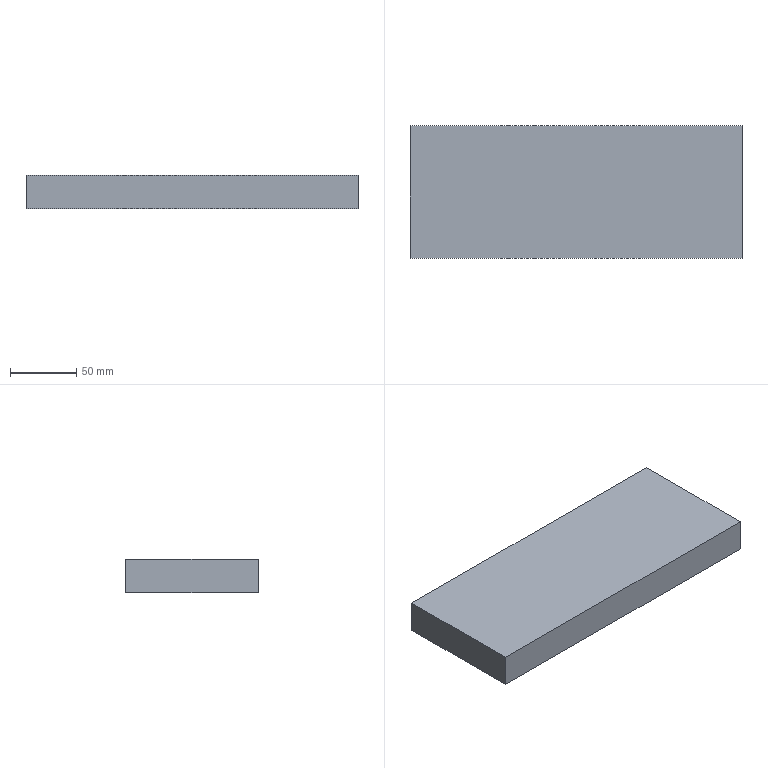Part | SolidWorks | features Extrusion 1 | 1 solid | 6 faces | box 250 x 100 x 25 mm | volume 625000 mm3 | plane 6
STEP:
#1=CARTESIAN_POINT('',(0.,0.,0.));
#2=VERTEX_POINT('',#1);
#3=CARTESIAN_POINT('',(0.,100.,0.));
#4=VERTEX_POINT('',#3);
#5=CARTESIAN_POINT('',(0.,0.,0.));
#6=DIRECTION('',(0.,1.,0.));
#7=VECTOR('',#6,1000.);
#8=LINE('',#5,#7);
#9=EDGE_CURVE('',#2,#4,#8,.T.);
#10=ORIENTED_EDGE('',*,*,#9,.T.);
#11=CARTESIAN_POINT('',(0.,100.,25.));
#12=VERTEX_POINT('',#11);
#13=CARTESIAN_POINT('',(0.,100.,25.));
#14=DIRECTION('',(0.,0.,-1.));
#15=VECTOR('',#14,1000.);
#16=LINE('',#13,#15);
#17=EDGE_CURVE('',#12,#4,#16,.T.);
#18=ORIENTED_EDGE('',*,*,#17,.F.);
#19=CARTESIAN_POINT('',(0.,0.,25.));
#20=VERTEX_POINT('',#19);
#21=CARTESIAN_POINT('',(0.,0.,25.));
#22=DIRECTION('',(0.,1.,0.));
#23=VECTOR('',#22,1000.);
#24=LINE('',#21,#23);
#25=EDGE_CURVE('',#20,#12,#24,.T.);
#26=ORIENTED_EDGE('',*,*,#25,.F.);
#27=CARTESIAN_POINT('',(0.,0.,25.));
#28=DIRECTION('',(0.,0.,-1.));
#29=VECTOR('',#28,1000.);
#30=LINE('',#27,#29);
#31=EDGE_CURVE('',#20,#2,#30,.T.);
#32=ORIENTED_EDGE('',*,*,#31,.T.);
#33=EDGE_LOOP('',(#10,#18,#26,#32));
#34=FACE_OUTER_BOUND('',#33,.T.);
#35=CARTESIAN_POINT('',(0.,0.,25.));
#36=DIRECTION('',(-1.,0.,0.));
#37=DIRECTION('',(0.,0.,1.));
#38=AXIS2_PLACEMENT_3D('',#35,#36,#37);
#39=PLANE('',#38);
#40=ADVANCED_FACE('',(#34),#39,.F.);
#41=CARTESIAN_POINT('',(-250.,100.,0.));
#42=VERTEX_POINT('',#41);
#43=CARTESIAN_POINT('',(0.,100.,0.));
#44=DIRECTION('',(-1.,0.,0.));
#45=VECTOR('',#44,1000.);
#46=LINE('',#43,#45);
#47=EDGE_CURVE('',#4,#42,#46,.T.);
#48=ORIENTED_EDGE('',*,*,#47,.T.);
#49=CARTESIAN_POINT('',(-250.,100.,25.));
#50=VERTEX_POINT('',#49);
#51=CARTESIAN_POINT('',(-250.,100.,25.));
#52=DIRECTION('',(0.,0.,-1.));
#53=VECTOR('',#52,1000.);
#54=LINE('',#51,#53);
#55=EDGE_CURVE('',#50,#42,#54,.T.);
#56=ORIENTED_EDGE('',*,*,#55,.F.);
#57=CARTESIAN_POINT('',(0.,100.,25.));
#58=DIRECTION('',(-1.,0.,0.));
#59=VECTOR('',#58,1000.);
#60=LINE('',#57,#59);
#61=EDGE_CURVE('',#12,#50,#60,.T.);
#62=ORIENTED_EDGE('',*,*,#61,.F.);
#63=ORIENTED_EDGE('',*,*,#17,.T.);
#64=EDGE_LOOP('',(#48,#56,#62,#63));
#65=FACE_OUTER_BOUND('',#64,.T.);
#66=CARTESIAN_POINT('',(0.,100.,25.));
#67=DIRECTION('',(0.,-1.,0.));
#68=DIRECTION('',(1.,0.,0.));
#69=AXIS2_PLACEMENT_3D('',#66,#67,#68);
#70=PLANE('',#69);
#71=ADVANCED_FACE('',(#65),#70,.F.);
#72=CARTESIAN_POINT('',(-250.,0.,0.));
#73=VERTEX_POINT('',#72);
#74=CARTESIAN_POINT('',(-250.,0.,0.));
#75=DIRECTION('',(0.,-1.,0.));
#76=VECTOR('',#75,1000.);
#77=LINE('',#74,#76);
#78=EDGE_CURVE('',#42,#73,#77,.T.);
#79=ORIENTED_EDGE('',*,*,#78,.T.);
#80=CARTESIAN_POINT('',(-250.,0.,25.));
#81=VERTEX_POINT('',#80);
#82=CARTESIAN_POINT('',(-250.,0.,25.));
#83=DIRECTION('',(0.,0.,-1.));
#84=VECTOR('',#83,1000.);
#85=LINE('',#82,#84);
#86=EDGE_CURVE('',#81,#73,#85,.T.);
#87=ORIENTED_EDGE('',*,*,#86,.F.);
#88=CARTESIAN_POINT('',(-250.,0.,25.));
#89=DIRECTION('',(0.,-1.,0.));
#90=VECTOR('',#89,1000.);
#91=LINE('',#88,#90);
#92=EDGE_CURVE('',#50,#81,#91,.T.);
#93=ORIENTED_EDGE('',*,*,#92,.F.);
#94=ORIENTED_EDGE('',*,*,#55,.T.);
#95=EDGE_LOOP('',(#79,#87,#93,#94));
#96=FACE_OUTER_BOUND('',#95,.T.);
#97=CARTESIAN_POINT('',(-250.,0.,25.));
#98=DIRECTION('',(1.,0.,0.));
#99=DIRECTION('',(0.,0.,-1.));
#100=AXIS2_PLACEMENT_3D('',#97,#98,#99);
#101=PLANE('',#100);
#102=ADVANCED_FACE('',(#96),#101,.F.);
#103=CARTESIAN_POINT('',(0.,0.,0.));
#104=DIRECTION('',(1.,0.,0.));
#105=VECTOR('',#104,1000.);
#106=LINE('',#103,#105);
#107=EDGE_CURVE('',#73,#2,#106,.T.);
#108=ORIENTED_EDGE('',*,*,#107,.T.);
#109=ORIENTED_EDGE('',*,*,#31,.F.);
#110=CARTESIAN_POINT('',(0.,0.,25.));
#111=DIRECTION('',(1.,0.,0.));
#112=VECTOR('',#111,1000.);
#113=LINE('',#110,#112);
#114=EDGE_CURVE('',#81,#20,#113,.T.);
#115=ORIENTED_EDGE('',*,*,#114,.F.);
#116=ORIENTED_EDGE('',*,*,#86,.T.);
#117=EDGE_LOOP('',(#108,#109,#115,#116));
#118=FACE_OUTER_BOUND('',#117,.T.);
#119=CARTESIAN_POINT('',(0.,0.,25.));
#120=DIRECTION('',(0.,1.,0.));
#121=DIRECTION('',(0.,0.,1.));
#122=AXIS2_PLACEMENT_3D('',#119,#120,#121);
#123=PLANE('',#122);
#124=ADVANCED_FACE('',(#118),#123,.F.);
#125=ORIENTED_EDGE('',*,*,#25,.T.);
#126=ORIENTED_EDGE('',*,*,#61,.T.);
#127=ORIENTED_EDGE('',*,*,#92,.T.);
#128=ORIENTED_EDGE('',*,*,#114,.T.);
#129=EDGE_LOOP('',(#125,#126,#127,#128));
#130=FACE_OUTER_BOUND('',#129,.T.);
#131=CARTESIAN_POINT('',(0.,0.,25.));
#132=DIRECTION('',(0.,0.,1.));
#133=DIRECTION('',(1.,0.,0.));
#134=AXIS2_PLACEMENT_3D('',#131,#132,#133);
#135=PLANE('',#134);
#136=ADVANCED_FACE('',(#130),#135,.T.);
#137=ORIENTED_EDGE('',*,*,#9,.F.);
#138=ORIENTED_EDGE('',*,*,#107,.F.);
#139=ORIENTED_EDGE('',*,*,#78,.F.);
#140=ORIENTED_EDGE('',*,*,#47,.F.);
#141=EDGE_LOOP('',(#137,#138,#139,#140));
#142=FACE_OUTER_BOUND('',#141,.T.);
#143=CARTESIAN_POINT('',(0.,0.,0.));
#144=DIRECTION('',(0.,0.,1.));
#145=DIRECTION('',(1.,0.,0.));
#146=AXIS2_PLACEMENT_3D('',#143,#144,#145);
#147=PLANE('',#146);
#148=ADVANCED_FACE('',(#142),#147,.F.);
#149=CLOSED_SHELL('',(#40,#71,#102,#124,#136,#148));
#150=MANIFOLD_SOLID_BREP('',#149);
#151=CARTESIAN_POINT('',(0.,0.,0.));
#152=DIRECTION('',(0.,0.,1.));
#153=DIRECTION('',(1.,0.,0.));
#154=AXIS2_PLACEMENT_3D('',#151,#152,#153);
#155=(LENGTH_UNIT()NAMED_UNIT(*)SI_UNIT(.MILLI.,.METRE.));
#156=UNCERTAINTY_MEASURE_WITH_UNIT(LENGTH_MEASURE(0.00001),#155,'','');
#157=(NAMED_UNIT(*)PLANE_ANGLE_UNIT()SI_UNIT($,.RADIAN.));
#158=(NAMED_UNIT(*)SI_UNIT($,.STERADIAN.)SOLID_ANGLE_UNIT());
#159=(GEOMETRIC_REPRESENTATION_CONTEXT(3)GLOBAL_UNCERTAINTY_ASSIGNED_CONTEXT((#156))GLOBAL_UNIT_ASSIGNED_CONTEXT((#155,#157,#158))REPRESENTATION_CONTEXT('',''));
#160=ADVANCED_BREP_SHAPE_REPRESENTATION('',(#150,#154),#159);